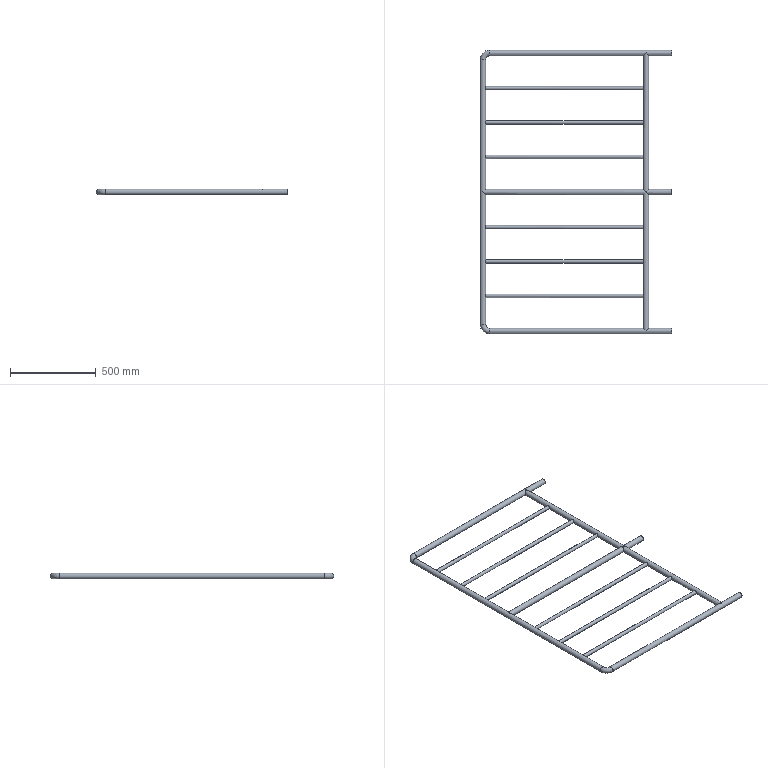Part | STEP file | PN_0005 guardrail 1620X1100 body_Default<As Machined> | 14 solids | 56 faces | box 1116 x 1652 x 32 mm | volume 1256893 mm3 | cylinder 41 | plane 11 | torus 4 | commonest cylinder face diameters 32 x23 18 x6 20 x6 29 x6